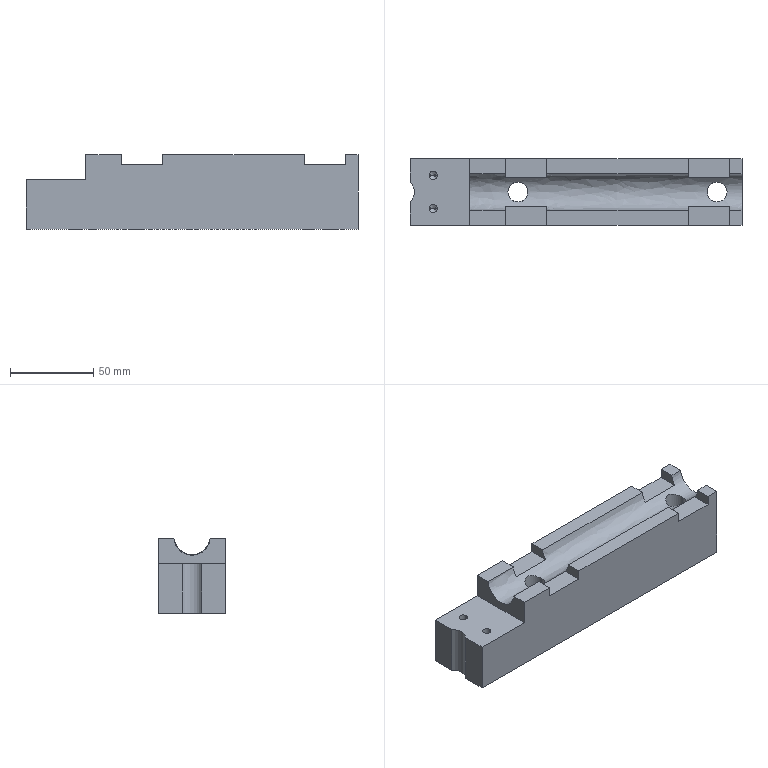NC program | NX | posted with a generic post
Whole program:
N10 G17 G21 G94 G90
(FLOOR_WALL_COPY , TOOL : D63)
N12 T01 M6
N14 G54
N16 G17 G0 G90 X-134.5 Y0. S6500 M3
N18 G43 Z30. H1
N20 Z7.
N22 G94 G1 Z4. F1250.
N24 X-131.5
N26 X131.5
N28 X134.5
N30 Z7.
N32 G0 Z30.
N34 X-134.5
N36 Z6.
N38 G1 Z3.
N40 X-131.5
N42 X131.5
N44 X134.5
N46 Z6.
N48 G0 Z30.
N50 X-134.5
N52 Z5.
N54 G1 Z2.
N56 X-131.5
N58 X131.5
N60 X134.5
N62 Z5.
N64 G0 Z30.
N66 X-134.5
N68 Z4.
N70 G1 Z1.
N72 X-131.5
N74 X131.5
N76 X134.5
N78 Z4.
N80 G0 Z30.
N82 X-134.5
N84 Z3.
N86 G1 Z0.
N88 X-131.5
N90 X131.5
N92 X134.5
N94 Z3.
N96 G0 Z30.
N98 M5
(DRILLING_COPY_1_COPY , TOOL : D6A45)
N100 T07 M6
N102 G54
N104 G17 G0 G90 X-85. Y0. S5000 M3
N106 G43 Z30. H7
N108 G94 G81 G98 Z-2.5 F250. R3.
N110 X-70. Y-12.5
N112 Y0.
N114 Y12.5
N116 X0.
N118 Y-12.5
N120 X35. Y0.
N122 X60.
N124 X70. Y-12.5
N126 Y12.5
N128 G80
N130 G0 X70. Y12.5 Z30.
N132 M5
(DRILLING_COPY_COPY_1_COPY_1 , TOOL : 4.8ZT)
N134 T14 M6
N136 G54
N138 G17 G0 G90 X-70. Y0. S2000 M3
N140 G43 Z30. H14
N142 G94 G83 G98 Z-13.442 F120. Q2. R3.
N144 X60.
N146 G80
N148 G0 X60. Y0. Z30.
N150 M5
(DRILLING_COPY_COPY_1_COPY_COPY , TOOL : 5.0JD)
N152 T15 M6
N154 G54
N156 G17 G0 G90 X-70. Y0. S1000 M3
N158 G43 Z30. H15
N160 G94 G85 G98 Z-12. F50. R3.
N162 X60.
N164 G80
N166 G0 X60. Y0. Z30.
N168 M5
(DRILLING_COPY_COPY_1_COPY_1_1 , TOOL : 7.0ZT)
N170 T17 M6
N172 G54
N174 G17 G0 G90 X-70. Y-12.5 S2000 M3
N176 G43 Z30. H17
N178 G94 G83 G98 Z-14.103 F200. Q2. R3.
N180 Y12.5
N182 X0.
N184 Y-12.5
N186 X70.
N188 Y12.5
N190 G80
N192 G0 X70. Y12.5 Z30.
N194 M5
(ZLEVEL_PROFILE_1_COPY_1_COPY_COPY_1 , TOOL : D6A45)
N196 T07 M6
N198 G54
N200 G17 G0 G90 X60.132 Y0.315 S9500 M3
N202 G43 Z30. H7
N204 Z0.
N206 G94 G1 Z-1. F1000.
N208 X60.52 Y1.241
N210 G3 X60. Y1.541 R0.6
N212 X58.459 Y0. R1.541
N214 X60. Y1.541 R-1.541
N216 X59.48 Y1.241 R0.6
N218 G1 X59.868 Y0.315
N220 Z0.
N222 G0 Z30.
N224 X-69.868
N226 Z0.
N228 G1 Z-1.
N230 X-69.48 Y1.241
N232 G3 X-70. Y1.541 R0.6
N234 X-71.541 Y0. R1.541
N236 X-70. Y1.541 R-1.541
N238 X-70.52 Y1.241 R0.6
N240 G1 X-70.132 Y0.315
N242 Z0.
N244 G0 Z30.
N246 X33.861 Y-3.669
N248 Z0.
N250 G1 Z-1.
N252 X34.48 Y-4.741
N254 G3 X35. Y-5.041 R0.6
N256 X40.041 Y0. R5.041
N258 X35. Y-5.041 R-5.041
N260 X35.52 Y-4.741 R0.6
N262 G1 X36.139 Y-3.669
N264 Z0.
N266 G0 Z30.
N268 X0.303 Y13.807
N270 Z0.
N272 G1 Z-1.
N274 X0.52 Y14.741
N276 G3 X0. Y15.041 R0.6
N278 X-2.541 Y12.5 R2.541
N280 X0. Y15.041 R-2.541
N282 X-0.52 Y14.741 R0.6
N284 G1 X-0.303 Y13.807
N286 Z0.
N288 G0 Z30.
N290 X-88.669 Y1.139
N292 Z0.
N294 G1 Z-1.
N296 X-89.741 Y0.52
N298 G3 X-90.041 Y0. R0.6
N300 G1 Y-0.003
N302 G3 X-84.997 Y-5.041 R5.041
N304 X-90.041 Y0. R-5.041
N306 X-89.741 Y-0.52 R0.6
N308 G1 X-88.669 Y-1.139
N310 Z0.
N312 G0 Z30.
N314 X-69.697 Y13.807
N316 Z0.
N318 G1 Z-1.
N320 X-69.48 Y14.741
N322 G3 X-70. Y15.041 R0.6
N324 X-72.541 Y12.5 R2.541
N326 X-70. Y15.041 R-2.541
N328 X-70.52 Y14.741 R0.6
N330 G1 X-70.303 Y13.807
N332 Z0.
N334 G0 Z30.
N336 X69.697 Y-13.807
N338 Z0.
N340 G1 Z-1.
N342 X69.48 Y-14.741
N344 G3 X70. Y-15.041 R0.6
N346 X72.541 Y-12.5 R2.541
N348 X70. Y-15.041 R-2.541
N350 X70.52 Y-14.741 R0.6
N352 G1 X70.303 Y-13.807
N354 Z0.
N356 G0 Z30.
N358 X-0.303
N360 Z0.
N362 G1 Z-1.
N364 X-0.52 Y-14.741
N366 G3 X0. Y-15.041 R0.6
N368 X2.541 Y-12.5 R2.541
N370 X0. Y-15.041 R-2.541
N372 X0.52 Y-14.741 R0.6
N374 G1 X0.303 Y-13.807
N376 Z0.
N378 G0 Z30.
N380 X-70.303
N382 Z0.
N384 G1 Z-1.
N386 X-70.52 Y-14.741
N388 G3 X-70. Y-15.041 R0.6
N390 X-67.459 Y-12.5 R2.541
N392 X-70. Y-15.041 R-2.541
N394 X-69.48 Y-14.741 R0.6
N396 G1 X-69.697 Y-13.807
N398 Z0.
N400 G0 Z30.
N402 X70.303 Y13.807
N404 Z0.
N406 G1 Z-1.
N408 X70.52 Y14.741
N410 G3 X70. Y15.041 R0.6
N412 X67.459 Y12.5 R2.541
N414 X70. Y15.041 R-2.541
N416 X69.48 Y14.741 R0.6
N418 G1 X69.697 Y13.807
N420 Z0.
N422 G0 Z30.
N424 X-100.921 Y21.952
N426 Z0.
N428 G1 Z-1.
N430 X-100.521 Y21.259
N432 G3 X-100.001 Y20.959 R0.6
N434 G1 X100.001
N436 G2 X100.959 Y20.001 R0.958
N438 G1 Y5.921
N440 G2 X100.619 Y5.189 R0.957
N442 G3 X100.619 Y-5.189 R6.791
N444 G2 X100.959 Y-5.921 R0.957
N446 G1 Y-20.001
N448 G2 X100.001 Y-20.959 R0.958
N450 G1 X-100.001
N452 G2 X-100.959 Y-20.001 R0.958
N454 G1 Y20.001
N456 G2 X-100.001 Y20.959 R0.958
N458 G3 X-99.481 Y21.259 R0.6
N460 G1 X-98.962 Y22.159
N462 Z0.
N464 G0 Z30.
N466 M5
N468 M2